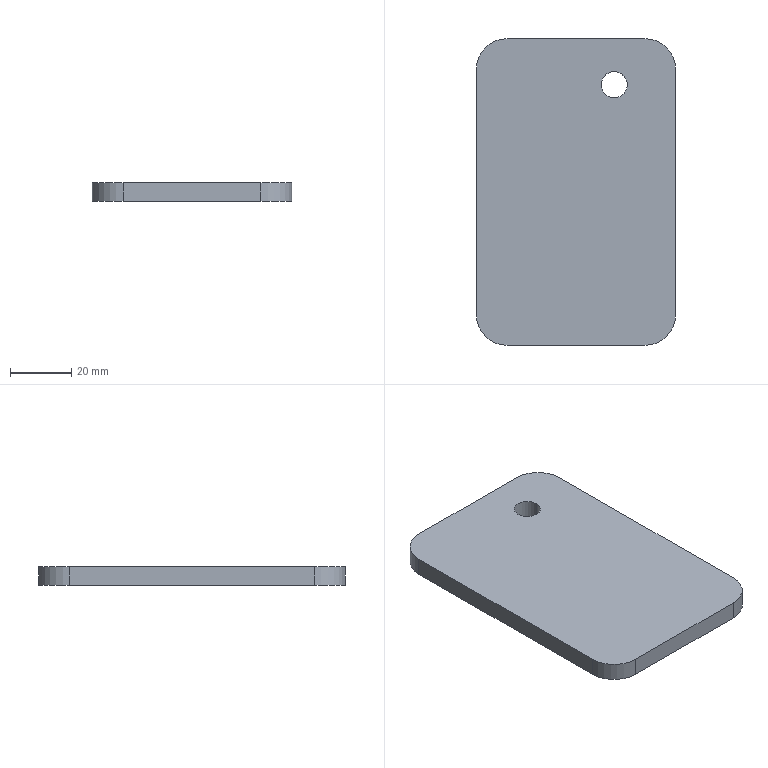Part | SolidWorks | features FlatPattern 1, SMBaseFlange 1, SheetMetal 1 | 1 solid | 12 faces | box 65 x 100 x 6 mm | volume 38144 mm3 | cylinder 6 | plane 6 | commonest cylinder face diameters 20 x4 8.5 x2
STEP:
#1=CARTESIAN_POINT('',(68.25,-500.5,6.));
#2=VERTEX_POINT('',#1);
#3=CARTESIAN_POINT('',(76.75,-500.5,6.));
#4=VERTEX_POINT('',#3);
#5=CARTESIAN_POINT('',(72.5,-500.5,6.));
#6=DIRECTION('',(0.,0.,1.));
#7=DIRECTION('',(1.,0.,0.));
#8=AXIS2_PLACEMENT_3D('',#5,#6,#7);
#9=CIRCLE('',#8,4.25);
#10=EDGE_CURVE('',#2,#4,#9,.T.);
#11=ORIENTED_EDGE('',*,*,#10,.T.);
#12=CARTESIAN_POINT('',(76.75,-500.5,0.));
#13=VERTEX_POINT('',#12);
#14=CARTESIAN_POINT('',(76.75,-500.5,6.));
#15=DIRECTION('',(0.,0.,-1.));
#16=VECTOR('',#15,1000.);
#17=LINE('',#14,#16);
#18=EDGE_CURVE('',#4,#13,#17,.T.);
#19=ORIENTED_EDGE('',*,*,#18,.T.);
#20=CARTESIAN_POINT('',(68.25,-500.5,0.));
#21=VERTEX_POINT('',#20);
#22=CARTESIAN_POINT('',(72.5,-500.5,0.));
#23=DIRECTION('',(0.,0.,1.));
#24=DIRECTION('',(1.,0.,0.));
#25=AXIS2_PLACEMENT_3D('',#22,#23,#24);
#26=CIRCLE('',#25,4.25);
#27=EDGE_CURVE('',#21,#13,#26,.T.);
#28=ORIENTED_EDGE('',*,*,#27,.F.);
#29=CARTESIAN_POINT('',(68.25,-500.5,6.));
#30=DIRECTION('',(0.,0.,-1.));
#31=VECTOR('',#30,1000.);
#32=LINE('',#29,#31);
#33=EDGE_CURVE('',#2,#21,#32,.T.);
#34=ORIENTED_EDGE('',*,*,#33,.F.);
#35=EDGE_LOOP('',(#11,#19,#28,#34));
#36=FACE_OUTER_BOUND('',#35,.T.);
#37=CARTESIAN_POINT('',(72.5,-500.5,6.));
#38=DIRECTION('',(0.,0.,-1.));
#39=DIRECTION('',(-1.,0.,0.));
#40=AXIS2_PLACEMENT_3D('',#37,#38,#39);
#41=CYLINDRICAL_SURFACE('',#40,4.25);
#42=ADVANCED_FACE('',(#36),#41,.F.);
#43=CARTESIAN_POINT('',(27.5,-575.5,6.));
#44=VERTEX_POINT('',#43);
#45=CARTESIAN_POINT('',(37.5,-585.5,6.));
#46=VERTEX_POINT('',#45);
#47=CARTESIAN_POINT('',(37.5,-575.5,6.));
#48=DIRECTION('',(0.,0.,1.));
#49=DIRECTION('',(1.,0.,0.));
#50=AXIS2_PLACEMENT_3D('',#47,#48,#49);
#51=CIRCLE('',#50,10.);
#52=EDGE_CURVE('',#44,#46,#51,.T.);
#53=ORIENTED_EDGE('',*,*,#52,.T.);
#54=CARTESIAN_POINT('',(82.5,-585.5,6.));
#55=VERTEX_POINT('',#54);
#56=CARTESIAN_POINT('',(37.5,-585.5,6.));
#57=DIRECTION('',(1.,0.,0.));
#58=VECTOR('',#57,1000.);
#59=LINE('',#56,#58);
#60=EDGE_CURVE('',#46,#55,#59,.T.);
#61=ORIENTED_EDGE('',*,*,#60,.T.);
#62=CARTESIAN_POINT('',(92.5,-575.5,6.));
#63=VERTEX_POINT('',#62);
#64=CARTESIAN_POINT('',(82.5,-575.5,6.));
#65=DIRECTION('',(0.,0.,1.));
#66=DIRECTION('',(1.,0.,0.));
#67=AXIS2_PLACEMENT_3D('',#64,#65,#66);
#68=CIRCLE('',#67,10.);
#69=EDGE_CURVE('',#55,#63,#68,.T.);
#70=ORIENTED_EDGE('',*,*,#69,.T.);
#71=CARTESIAN_POINT('',(92.5,-495.5,6.));
#72=VERTEX_POINT('',#71);
#73=CARTESIAN_POINT('',(92.5,-495.5,6.));
#74=DIRECTION('',(0.,1.,0.));
#75=VECTOR('',#74,1000.);
#76=LINE('',#73,#75);
#77=EDGE_CURVE('',#63,#72,#76,.T.);
#78=ORIENTED_EDGE('',*,*,#77,.T.);
#79=CARTESIAN_POINT('',(82.5,-485.5,6.));
#80=VERTEX_POINT('',#79);
#81=CARTESIAN_POINT('',(82.5,-495.5,6.));
#82=DIRECTION('',(0.,0.,1.));
#83=DIRECTION('',(-1.,0.,0.));
#84=AXIS2_PLACEMENT_3D('',#81,#82,#83);
#85=CIRCLE('',#84,10.);
#86=EDGE_CURVE('',#72,#80,#85,.T.);
#87=ORIENTED_EDGE('',*,*,#86,.T.);
#88=CARTESIAN_POINT('',(37.5,-485.5,6.));
#89=VERTEX_POINT('',#88);
#90=CARTESIAN_POINT('',(37.5,-485.5,6.));
#91=DIRECTION('',(-1.,0.,0.));
#92=VECTOR('',#91,1000.);
#93=LINE('',#90,#92);
#94=EDGE_CURVE('',#80,#89,#93,.T.);
#95=ORIENTED_EDGE('',*,*,#94,.T.);
#96=CARTESIAN_POINT('',(27.5,-495.5,6.));
#97=VERTEX_POINT('',#96);
#98=CARTESIAN_POINT('',(37.5,-495.5,6.));
#99=DIRECTION('',(0.,0.,1.));
#100=DIRECTION('',(1.,0.,0.));
#101=AXIS2_PLACEMENT_3D('',#98,#99,#100);
#102=CIRCLE('',#101,10.);
#103=EDGE_CURVE('',#89,#97,#102,.T.);
#104=ORIENTED_EDGE('',*,*,#103,.T.);
#105=CARTESIAN_POINT('',(27.5,-495.5,6.));
#106=DIRECTION('',(0.,-1.,0.));
#107=VECTOR('',#106,1000.);
#108=LINE('',#105,#107);
#109=EDGE_CURVE('',#97,#44,#108,.T.);
#110=ORIENTED_EDGE('',*,*,#109,.T.);
#111=EDGE_LOOP('',(#53,#61,#70,#78,#87,#95,#104,#110));
#112=FACE_OUTER_BOUND('',#111,.T.);
#113=ORIENTED_EDGE('',*,*,#10,.F.);
#114=CARTESIAN_POINT('',(72.5,-500.5,6.));
#115=DIRECTION('',(0.,0.,1.));
#116=DIRECTION('',(1.,0.,0.));
#117=AXIS2_PLACEMENT_3D('',#114,#115,#116);
#118=CIRCLE('',#117,4.25);
#119=EDGE_CURVE('',#4,#2,#118,.T.);
#120=ORIENTED_EDGE('',*,*,#119,.F.);
#121=EDGE_LOOP('',(#113,#120));
#122=FACE_BOUND('',#121,.T.);
#123=CARTESIAN_POINT('',(37.5,-575.5,6.));
#124=DIRECTION('',(0.,0.,1.));
#125=DIRECTION('',(1.,0.,0.));
#126=AXIS2_PLACEMENT_3D('',#123,#124,#125);
#127=PLANE('',#126);
#128=ADVANCED_FACE('',(#112,#122),#127,.T.);
#129=CARTESIAN_POINT('',(27.5,-575.5,0.));
#130=VERTEX_POINT('',#129);
#131=CARTESIAN_POINT('',(37.5,-585.5,0.));
#132=VERTEX_POINT('',#131);
#133=CARTESIAN_POINT('',(37.5,-575.5,0.));
#134=DIRECTION('',(0.,0.,1.));
#135=DIRECTION('',(1.,0.,0.));
#136=AXIS2_PLACEMENT_3D('',#133,#134,#135);
#137=CIRCLE('',#136,10.);
#138=EDGE_CURVE('',#130,#132,#137,.T.);
#139=ORIENTED_EDGE('',*,*,#138,.F.);
#140=CARTESIAN_POINT('',(27.5,-495.5,0.));
#141=VERTEX_POINT('',#140);
#142=CARTESIAN_POINT('',(27.5,-495.5,0.));
#143=DIRECTION('',(0.,-1.,0.));
#144=VECTOR('',#143,1000.);
#145=LINE('',#142,#144);
#146=EDGE_CURVE('',#141,#130,#145,.T.);
#147=ORIENTED_EDGE('',*,*,#146,.F.);
#148=CARTESIAN_POINT('',(37.5,-485.5,0.));
#149=VERTEX_POINT('',#148);
#150=CARTESIAN_POINT('',(37.5,-495.5,0.));
#151=DIRECTION('',(0.,0.,1.));
#152=DIRECTION('',(1.,0.,0.));
#153=AXIS2_PLACEMENT_3D('',#150,#151,#152);
#154=CIRCLE('',#153,10.);
#155=EDGE_CURVE('',#149,#141,#154,.T.);
#156=ORIENTED_EDGE('',*,*,#155,.F.);
#157=CARTESIAN_POINT('',(82.5,-485.5,0.));
#158=VERTEX_POINT('',#157);
#159=CARTESIAN_POINT('',(37.5,-485.5,0.));
#160=DIRECTION('',(-1.,0.,0.));
#161=VECTOR('',#160,1000.);
#162=LINE('',#159,#161);
#163=EDGE_CURVE('',#158,#149,#162,.T.);
#164=ORIENTED_EDGE('',*,*,#163,.F.);
#165=CARTESIAN_POINT('',(92.5,-495.5,0.));
#166=VERTEX_POINT('',#165);
#167=CARTESIAN_POINT('',(82.5,-495.5,0.));
#168=DIRECTION('',(0.,0.,1.));
#169=DIRECTION('',(-1.,0.,0.));
#170=AXIS2_PLACEMENT_3D('',#167,#168,#169);
#171=CIRCLE('',#170,10.);
#172=EDGE_CURVE('',#166,#158,#171,.T.);
#173=ORIENTED_EDGE('',*,*,#172,.F.);
#174=CARTESIAN_POINT('',(92.5,-575.5,0.));
#175=VERTEX_POINT('',#174);
#176=CARTESIAN_POINT('',(92.5,-495.5,0.));
#177=DIRECTION('',(0.,1.,0.));
#178=VECTOR('',#177,1000.);
#179=LINE('',#176,#178);
#180=EDGE_CURVE('',#175,#166,#179,.T.);
#181=ORIENTED_EDGE('',*,*,#180,.F.);
#182=CARTESIAN_POINT('',(82.5,-585.5,0.));
#183=VERTEX_POINT('',#182);
#184=CARTESIAN_POINT('',(82.5,-575.5,0.));
#185=DIRECTION('',(0.,0.,1.));
#186=DIRECTION('',(1.,0.,0.));
#187=AXIS2_PLACEMENT_3D('',#184,#185,#186);
#188=CIRCLE('',#187,10.);
#189=EDGE_CURVE('',#183,#175,#188,.T.);
#190=ORIENTED_EDGE('',*,*,#189,.F.);
#191=CARTESIAN_POINT('',(37.5,-585.5,0.));
#192=DIRECTION('',(1.,0.,0.));
#193=VECTOR('',#192,1000.);
#194=LINE('',#191,#193);
#195=EDGE_CURVE('',#132,#183,#194,.T.);
#196=ORIENTED_EDGE('',*,*,#195,.F.);
#197=EDGE_LOOP('',(#139,#147,#156,#164,#173,#181,#190,#196));
#198=FACE_OUTER_BOUND('',#197,.T.);
#199=ORIENTED_EDGE('',*,*,#27,.T.);
#200=CARTESIAN_POINT('',(72.5,-500.5,0.));
#201=DIRECTION('',(0.,0.,1.));
#202=DIRECTION('',(1.,0.,0.));
#203=AXIS2_PLACEMENT_3D('',#200,#201,#202);
#204=CIRCLE('',#203,4.25);
#205=EDGE_CURVE('',#13,#21,#204,.T.);
#206=ORIENTED_EDGE('',*,*,#205,.T.);
#207=EDGE_LOOP('',(#199,#206));
#208=FACE_BOUND('',#207,.T.);
#209=CARTESIAN_POINT('',(37.5,-575.5,0.));
#210=DIRECTION('',(0.,0.,1.));
#211=DIRECTION('',(1.,0.,0.));
#212=AXIS2_PLACEMENT_3D('',#209,#210,#211);
#213=PLANE('',#212);
#214=ADVANCED_FACE('',(#198,#208),#213,.F.);
#215=ORIENTED_EDGE('',*,*,#138,.T.);
#216=CARTESIAN_POINT('',(37.5,-585.5,6.));
#217=DIRECTION('',(0.,0.,-1.));
#218=VECTOR('',#217,1000.);
#219=LINE('',#216,#218);
#220=EDGE_CURVE('',#46,#132,#219,.T.);
#221=ORIENTED_EDGE('',*,*,#220,.F.);
#222=ORIENTED_EDGE('',*,*,#52,.F.);
#223=CARTESIAN_POINT('',(27.5,-575.5,6.));
#224=DIRECTION('',(0.,0.,-1.));
#225=VECTOR('',#224,1000.);
#226=LINE('',#223,#225);
#227=EDGE_CURVE('',#44,#130,#226,.T.);
#228=ORIENTED_EDGE('',*,*,#227,.T.);
#229=EDGE_LOOP('',(#215,#221,#222,#228));
#230=FACE_OUTER_BOUND('',#229,.T.);
#231=CARTESIAN_POINT('',(37.5,-575.5,6.));
#232=DIRECTION('',(0.,0.,-1.));
#233=DIRECTION('',(-1.,0.,0.));
#234=AXIS2_PLACEMENT_3D('',#231,#232,#233);
#235=CYLINDRICAL_SURFACE('',#234,10.);
#236=ADVANCED_FACE('',(#230),#235,.T.);
#237=ORIENTED_EDGE('',*,*,#195,.T.);
#238=CARTESIAN_POINT('',(82.5,-585.5,6.));
#239=DIRECTION('',(0.,0.,-1.));
#240=VECTOR('',#239,1000.);
#241=LINE('',#238,#240);
#242=EDGE_CURVE('',#55,#183,#241,.T.);
#243=ORIENTED_EDGE('',*,*,#242,.F.);
#244=ORIENTED_EDGE('',*,*,#60,.F.);
#245=ORIENTED_EDGE('',*,*,#220,.T.);
#246=EDGE_LOOP('',(#237,#243,#244,#245));
#247=FACE_OUTER_BOUND('',#246,.T.);
#248=CARTESIAN_POINT('',(37.5,-585.5,6.));
#249=DIRECTION('',(0.,1.,0.));
#250=DIRECTION('',(0.,0.,1.));
#251=AXIS2_PLACEMENT_3D('',#248,#249,#250);
#252=PLANE('',#251);
#253=ADVANCED_FACE('',(#247),#252,.F.);
#254=ORIENTED_EDGE('',*,*,#189,.T.);
#255=CARTESIAN_POINT('',(92.5,-575.5,6.));
#256=DIRECTION('',(0.,0.,-1.));
#257=VECTOR('',#256,1000.);
#258=LINE('',#255,#257);
#259=EDGE_CURVE('',#63,#175,#258,.T.);
#260=ORIENTED_EDGE('',*,*,#259,.F.);
#261=ORIENTED_EDGE('',*,*,#69,.F.);
#262=ORIENTED_EDGE('',*,*,#242,.T.);
#263=EDGE_LOOP('',(#254,#260,#261,#262));
#264=FACE_OUTER_BOUND('',#263,.T.);
#265=CARTESIAN_POINT('',(82.5,-575.5,6.));
#266=DIRECTION('',(0.,0.,-1.));
#267=DIRECTION('',(-1.,0.,0.));
#268=AXIS2_PLACEMENT_3D('',#265,#266,#267);
#269=CYLINDRICAL_SURFACE('',#268,10.);
#270=ADVANCED_FACE('',(#264),#269,.T.);
#271=ORIENTED_EDGE('',*,*,#180,.T.);
#272=CARTESIAN_POINT('',(92.5,-495.5,6.));
#273=DIRECTION('',(0.,0.,-1.));
#274=VECTOR('',#273,1000.);
#275=LINE('',#272,#274);
#276=EDGE_CURVE('',#72,#166,#275,.T.);
#277=ORIENTED_EDGE('',*,*,#276,.F.);
#278=ORIENTED_EDGE('',*,*,#77,.F.);
#279=ORIENTED_EDGE('',*,*,#259,.T.);
#280=EDGE_LOOP('',(#271,#277,#278,#279));
#281=FACE_OUTER_BOUND('',#280,.T.);
#282=CARTESIAN_POINT('',(92.5,-495.5,6.));
#283=DIRECTION('',(-1.,0.,0.));
#284=DIRECTION('',(0.,0.,1.));
#285=AXIS2_PLACEMENT_3D('',#282,#283,#284);
#286=PLANE('',#285);
#287=ADVANCED_FACE('',(#281),#286,.F.);
#288=ORIENTED_EDGE('',*,*,#172,.T.);
#289=CARTESIAN_POINT('',(82.5,-485.5,6.));
#290=DIRECTION('',(0.,0.,-1.));
#291=VECTOR('',#290,1000.);
#292=LINE('',#289,#291);
#293=EDGE_CURVE('',#80,#158,#292,.T.);
#294=ORIENTED_EDGE('',*,*,#293,.F.);
#295=ORIENTED_EDGE('',*,*,#86,.F.);
#296=ORIENTED_EDGE('',*,*,#276,.T.);
#297=EDGE_LOOP('',(#288,#294,#295,#296));
#298=FACE_OUTER_BOUND('',#297,.T.);
#299=CARTESIAN_POINT('',(82.5,-495.5,6.));
#300=DIRECTION('',(0.,0.,-1.));
#301=DIRECTION('',(-1.,0.,0.));
#302=AXIS2_PLACEMENT_3D('',#299,#300,#301);
#303=CYLINDRICAL_SURFACE('',#302,10.);
#304=ADVANCED_FACE('',(#298),#303,.T.);
#305=ORIENTED_EDGE('',*,*,#163,.T.);
#306=CARTESIAN_POINT('',(37.5,-485.5,6.));
#307=DIRECTION('',(0.,0.,-1.));
#308=VECTOR('',#307,1000.);
#309=LINE('',#306,#308);
#310=EDGE_CURVE('',#89,#149,#309,.T.);
#311=ORIENTED_EDGE('',*,*,#310,.F.);
#312=ORIENTED_EDGE('',*,*,#94,.F.);
#313=ORIENTED_EDGE('',*,*,#293,.T.);
#314=EDGE_LOOP('',(#305,#311,#312,#313));
#315=FACE_OUTER_BOUND('',#314,.T.);
#316=CARTESIAN_POINT('',(37.5,-485.5,6.));
#317=DIRECTION('',(0.,-1.,0.));
#318=DIRECTION('',(1.,0.,0.));
#319=AXIS2_PLACEMENT_3D('',#316,#317,#318);
#320=PLANE('',#319);
#321=ADVANCED_FACE('',(#315),#320,.F.);
#322=ORIENTED_EDGE('',*,*,#155,.T.);
#323=CARTESIAN_POINT('',(27.5,-495.5,6.));
#324=DIRECTION('',(0.,0.,-1.));
#325=VECTOR('',#324,1000.);
#326=LINE('',#323,#325);
#327=EDGE_CURVE('',#97,#141,#326,.T.);
#328=ORIENTED_EDGE('',*,*,#327,.F.);
#329=ORIENTED_EDGE('',*,*,#103,.F.);
#330=ORIENTED_EDGE('',*,*,#310,.T.);
#331=EDGE_LOOP('',(#322,#328,#329,#330));
#332=FACE_OUTER_BOUND('',#331,.T.);
#333=CARTESIAN_POINT('',(37.5,-495.5,6.));
#334=DIRECTION('',(0.,0.,-1.));
#335=DIRECTION('',(-1.,0.,0.));
#336=AXIS2_PLACEMENT_3D('',#333,#334,#335);
#337=CYLINDRICAL_SURFACE('',#336,10.);
#338=ADVANCED_FACE('',(#332),#337,.T.);
#339=ORIENTED_EDGE('',*,*,#146,.T.);
#340=ORIENTED_EDGE('',*,*,#227,.F.);
#341=ORIENTED_EDGE('',*,*,#109,.F.);
#342=ORIENTED_EDGE('',*,*,#327,.T.);
#343=EDGE_LOOP('',(#339,#340,#341,#342));
#344=FACE_OUTER_BOUND('',#343,.T.);
#345=CARTESIAN_POINT('',(27.5,-495.5,6.));
#346=DIRECTION('',(1.,0.,0.));
#347=DIRECTION('',(0.,1.,0.));
#348=AXIS2_PLACEMENT_3D('',#345,#346,#347);
#349=PLANE('',#348);
#350=ADVANCED_FACE('',(#344),#349,.F.);
#351=ORIENTED_EDGE('',*,*,#18,.F.);
#352=ORIENTED_EDGE('',*,*,#119,.T.);
#353=ORIENTED_EDGE('',*,*,#33,.T.);
#354=ORIENTED_EDGE('',*,*,#205,.F.);
#355=EDGE_LOOP('',(#351,#352,#353,#354));
#356=FACE_OUTER_BOUND('',#355,.T.);
#357=CARTESIAN_POINT('',(72.5,-500.5,6.));
#358=DIRECTION('',(0.,0.,-1.));
#359=DIRECTION('',(-1.,0.,0.));
#360=AXIS2_PLACEMENT_3D('',#357,#358,#359);
#361=CYLINDRICAL_SURFACE('',#360,4.25);
#362=ADVANCED_FACE('',(#356),#361,.F.);
#363=CLOSED_SHELL('',(#42,#128,#214,#236,#253,#270,#287,#304,#321,#338,#350,#362));
#364=MANIFOLD_SOLID_BREP('',#363);
#365=CARTESIAN_POINT('',(0.,0.,0.));
#366=DIRECTION('',(0.,0.,1.));
#367=DIRECTION('',(1.,0.,0.));
#368=AXIS2_PLACEMENT_3D('',#365,#366,#367);
#369=(LENGTH_UNIT()NAMED_UNIT(*)SI_UNIT(.MILLI.,.METRE.));
#370=UNCERTAINTY_MEASURE_WITH_UNIT(LENGTH_MEASURE(0.00001),#369,'','');
#371=(NAMED_UNIT(*)PLANE_ANGLE_UNIT()SI_UNIT($,.RADIAN.));
#372=(NAMED_UNIT(*)SI_UNIT($,.STERADIAN.)SOLID_ANGLE_UNIT());
#373=(GEOMETRIC_REPRESENTATION_CONTEXT(3)GLOBAL_UNCERTAINTY_ASSIGNED_CONTEXT((#370))GLOBAL_UNIT_ASSIGNED_CONTEXT((#369,#371,#372))REPRESENTATION_CONTEXT('',''));
#374=ADVANCED_BREP_SHAPE_REPRESENTATION('',(#364,#368),#373);